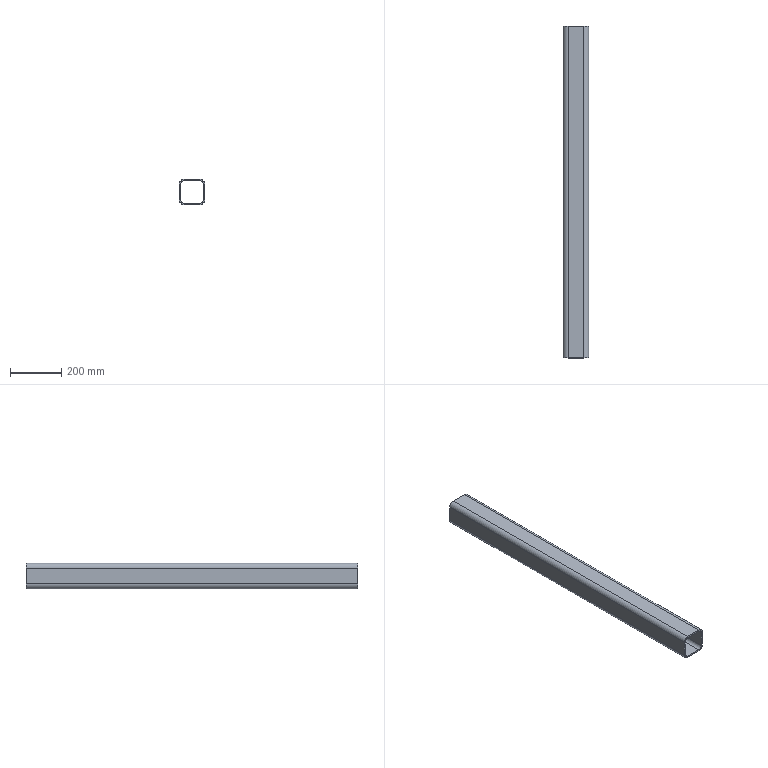Part | SolidWorks | features WeldMemberFeat 1, WeldmentFeature 1 | 1 solid | 18 faces | box 100 x 1293 x 100 mm | volume 2703104 mm3 | plane 10 | cylinder 8 | commonest cylinder face diameters 26.12 x4 38.12 x4
STEP:
#1=CARTESIAN_POINT('',(50.,1293.,30.94));
#2=VERTEX_POINT('',#1);
#3=CARTESIAN_POINT('',(30.94,1293.,50.));
#4=VERTEX_POINT('',#3);
#5=CARTESIAN_POINT('',(30.94,1293.,30.94));
#6=DIRECTION('',(0.,-1.,0.));
#7=DIRECTION('',(1.,0.,0.));
#8=AXIS2_PLACEMENT_3D('',#5,#6,#7);
#9=CIRCLE('',#8,19.06);
#10=EDGE_CURVE('',#2,#4,#9,.T.);
#11=ORIENTED_EDGE('',*,*,#10,.T.);
#12=CARTESIAN_POINT('',(30.94,0.,50.));
#13=VERTEX_POINT('',#12);
#14=CARTESIAN_POINT('',(30.94,0.,50.));
#15=DIRECTION('',(0.,1.,0.));
#16=VECTOR('',#15,1000.);
#17=LINE('',#14,#16);
#18=EDGE_CURVE('',#13,#4,#17,.T.);
#19=ORIENTED_EDGE('',*,*,#18,.F.);
#20=CARTESIAN_POINT('',(50.,0.,30.94));
#21=VERTEX_POINT('',#20);
#22=CARTESIAN_POINT('',(30.94,0.,30.94));
#23=DIRECTION('',(0.,-1.,0.));
#24=DIRECTION('',(1.,0.,0.));
#25=AXIS2_PLACEMENT_3D('',#22,#23,#24);
#26=CIRCLE('',#25,19.06);
#27=EDGE_CURVE('',#21,#13,#26,.T.);
#28=ORIENTED_EDGE('',*,*,#27,.F.);
#29=CARTESIAN_POINT('',(50.,0.,30.94));
#30=DIRECTION('',(0.,1.,0.));
#31=VECTOR('',#30,1000.);
#32=LINE('',#29,#31);
#33=EDGE_CURVE('',#21,#2,#32,.T.);
#34=ORIENTED_EDGE('',*,*,#33,.T.);
#35=EDGE_LOOP('',(#11,#19,#28,#34));
#36=FACE_OUTER_BOUND('',#35,.T.);
#37=CARTESIAN_POINT('',(30.94,0.,30.94));
#38=DIRECTION('',(0.,1.,0.));
#39=DIRECTION('',(-1.,0.,0.));
#40=AXIS2_PLACEMENT_3D('',#37,#38,#39);
#41=CYLINDRICAL_SURFACE('',#40,19.06);
#42=ADVANCED_FACE('',(#36),#41,.T.);
#43=CARTESIAN_POINT('',(-30.94,1293.,50.));
#44=VERTEX_POINT('',#43);
#45=CARTESIAN_POINT('',(30.94,1293.,50.));
#46=DIRECTION('',(-1.,0.,0.));
#47=VECTOR('',#46,1000.);
#48=LINE('',#45,#47);
#49=EDGE_CURVE('',#4,#44,#48,.T.);
#50=ORIENTED_EDGE('',*,*,#49,.T.);
#51=CARTESIAN_POINT('',(-30.94,0.,50.));
#52=VERTEX_POINT('',#51);
#53=CARTESIAN_POINT('',(-30.94,0.,50.));
#54=DIRECTION('',(0.,1.,0.));
#55=VECTOR('',#54,1000.);
#56=LINE('',#53,#55);
#57=EDGE_CURVE('',#52,#44,#56,.T.);
#58=ORIENTED_EDGE('',*,*,#57,.F.);
#59=CARTESIAN_POINT('',(30.94,0.,50.));
#60=DIRECTION('',(-1.,0.,0.));
#61=VECTOR('',#60,1000.);
#62=LINE('',#59,#61);
#63=EDGE_CURVE('',#13,#52,#62,.T.);
#64=ORIENTED_EDGE('',*,*,#63,.F.);
#65=ORIENTED_EDGE('',*,*,#18,.T.);
#66=EDGE_LOOP('',(#50,#58,#64,#65));
#67=FACE_OUTER_BOUND('',#66,.T.);
#68=CARTESIAN_POINT('',(30.94,0.,50.));
#69=DIRECTION('',(0.,0.,-1.));
#70=DIRECTION('',(-1.,0.,0.));
#71=AXIS2_PLACEMENT_3D('',#68,#69,#70);
#72=PLANE('',#71);
#73=ADVANCED_FACE('',(#67),#72,.F.);
#74=CARTESIAN_POINT('',(-50.,1293.,30.94));
#75=VERTEX_POINT('',#74);
#76=CARTESIAN_POINT('',(-30.94,1293.,30.94));
#77=DIRECTION('',(0.,-1.,0.));
#78=DIRECTION('',(1.,0.,0.));
#79=AXIS2_PLACEMENT_3D('',#76,#77,#78);
#80=CIRCLE('',#79,19.06);
#81=EDGE_CURVE('',#44,#75,#80,.T.);
#82=ORIENTED_EDGE('',*,*,#81,.T.);
#83=CARTESIAN_POINT('',(-50.,0.,30.94));
#84=VERTEX_POINT('',#83);
#85=CARTESIAN_POINT('',(-50.,0.,30.94));
#86=DIRECTION('',(0.,1.,0.));
#87=VECTOR('',#86,1000.);
#88=LINE('',#85,#87);
#89=EDGE_CURVE('',#84,#75,#88,.T.);
#90=ORIENTED_EDGE('',*,*,#89,.F.);
#91=CARTESIAN_POINT('',(-30.94,0.,30.94));
#92=DIRECTION('',(0.,-1.,0.));
#93=DIRECTION('',(1.,0.,0.));
#94=AXIS2_PLACEMENT_3D('',#91,#92,#93);
#95=CIRCLE('',#94,19.06);
#96=EDGE_CURVE('',#52,#84,#95,.T.);
#97=ORIENTED_EDGE('',*,*,#96,.F.);
#98=ORIENTED_EDGE('',*,*,#57,.T.);
#99=EDGE_LOOP('',(#82,#90,#97,#98));
#100=FACE_OUTER_BOUND('',#99,.T.);
#101=CARTESIAN_POINT('',(-30.94,0.,30.94));
#102=DIRECTION('',(0.,1.,0.));
#103=DIRECTION('',(-1.,0.,0.));
#104=AXIS2_PLACEMENT_3D('',#101,#102,#103);
#105=CYLINDRICAL_SURFACE('',#104,19.06);
#106=ADVANCED_FACE('',(#100),#105,.T.);
#107=CARTESIAN_POINT('',(-50.,1293.,-30.94));
#108=VERTEX_POINT('',#107);
#109=CARTESIAN_POINT('',(-50.,1293.,-30.94));
#110=DIRECTION('',(0.,0.,-1.));
#111=VECTOR('',#110,1000.);
#112=LINE('',#109,#111);
#113=EDGE_CURVE('',#75,#108,#112,.T.);
#114=ORIENTED_EDGE('',*,*,#113,.T.);
#115=CARTESIAN_POINT('',(-50.,0.,-30.94));
#116=VERTEX_POINT('',#115);
#117=CARTESIAN_POINT('',(-50.,0.,-30.94));
#118=DIRECTION('',(0.,1.,0.));
#119=VECTOR('',#118,1000.);
#120=LINE('',#117,#119);
#121=EDGE_CURVE('',#116,#108,#120,.T.);
#122=ORIENTED_EDGE('',*,*,#121,.F.);
#123=CARTESIAN_POINT('',(-50.,0.,-30.94));
#124=DIRECTION('',(0.,0.,-1.));
#125=VECTOR('',#124,1000.);
#126=LINE('',#123,#125);
#127=EDGE_CURVE('',#84,#116,#126,.T.);
#128=ORIENTED_EDGE('',*,*,#127,.F.);
#129=ORIENTED_EDGE('',*,*,#89,.T.);
#130=EDGE_LOOP('',(#114,#122,#128,#129));
#131=FACE_OUTER_BOUND('',#130,.T.);
#132=CARTESIAN_POINT('',(-50.,0.,-30.94));
#133=DIRECTION('',(1.,0.,0.));
#134=DIRECTION('',(0.,0.,-1.));
#135=AXIS2_PLACEMENT_3D('',#132,#133,#134);
#136=PLANE('',#135);
#137=ADVANCED_FACE('',(#131),#136,.F.);
#138=CARTESIAN_POINT('',(-30.94,1293.,-50.));
#139=VERTEX_POINT('',#138);
#140=CARTESIAN_POINT('',(-30.94,1293.,-30.94));
#141=DIRECTION('',(0.,-1.,0.));
#142=DIRECTION('',(1.,0.,0.));
#143=AXIS2_PLACEMENT_3D('',#140,#141,#142);
#144=CIRCLE('',#143,19.06);
#145=EDGE_CURVE('',#108,#139,#144,.T.);
#146=ORIENTED_EDGE('',*,*,#145,.T.);
#147=CARTESIAN_POINT('',(-30.94,0.,-50.));
#148=VERTEX_POINT('',#147);
#149=CARTESIAN_POINT('',(-30.94,0.,-50.));
#150=DIRECTION('',(0.,1.,0.));
#151=VECTOR('',#150,1000.);
#152=LINE('',#149,#151);
#153=EDGE_CURVE('',#148,#139,#152,.T.);
#154=ORIENTED_EDGE('',*,*,#153,.F.);
#155=CARTESIAN_POINT('',(-30.94,0.,-30.94));
#156=DIRECTION('',(0.,-1.,0.));
#157=DIRECTION('',(1.,0.,0.));
#158=AXIS2_PLACEMENT_3D('',#155,#156,#157);
#159=CIRCLE('',#158,19.06);
#160=EDGE_CURVE('',#116,#148,#159,.T.);
#161=ORIENTED_EDGE('',*,*,#160,.F.);
#162=ORIENTED_EDGE('',*,*,#121,.T.);
#163=EDGE_LOOP('',(#146,#154,#161,#162));
#164=FACE_OUTER_BOUND('',#163,.T.);
#165=CARTESIAN_POINT('',(-30.94,0.,-30.94));
#166=DIRECTION('',(0.,1.,0.));
#167=DIRECTION('',(-1.,0.,0.));
#168=AXIS2_PLACEMENT_3D('',#165,#166,#167);
#169=CYLINDRICAL_SURFACE('',#168,19.06);
#170=ADVANCED_FACE('',(#164),#169,.T.);
#171=CARTESIAN_POINT('',(30.94,1293.,-50.));
#172=VERTEX_POINT('',#171);
#173=CARTESIAN_POINT('',(-30.94,1293.,-50.));
#174=DIRECTION('',(1.,0.,0.));
#175=VECTOR('',#174,1000.);
#176=LINE('',#173,#175);
#177=EDGE_CURVE('',#139,#172,#176,.T.);
#178=ORIENTED_EDGE('',*,*,#177,.T.);
#179=CARTESIAN_POINT('',(30.94,0.,-50.));
#180=VERTEX_POINT('',#179);
#181=CARTESIAN_POINT('',(30.94,0.,-50.));
#182=DIRECTION('',(0.,1.,0.));
#183=VECTOR('',#182,1000.);
#184=LINE('',#181,#183);
#185=EDGE_CURVE('',#180,#172,#184,.T.);
#186=ORIENTED_EDGE('',*,*,#185,.F.);
#187=CARTESIAN_POINT('',(-30.94,0.,-50.));
#188=DIRECTION('',(1.,0.,0.));
#189=VECTOR('',#188,1000.);
#190=LINE('',#187,#189);
#191=EDGE_CURVE('',#148,#180,#190,.T.);
#192=ORIENTED_EDGE('',*,*,#191,.F.);
#193=ORIENTED_EDGE('',*,*,#153,.T.);
#194=EDGE_LOOP('',(#178,#186,#192,#193));
#195=FACE_OUTER_BOUND('',#194,.T.);
#196=CARTESIAN_POINT('',(-30.94,0.,-50.));
#197=DIRECTION('',(0.,0.,1.));
#198=DIRECTION('',(1.,0.,0.));
#199=AXIS2_PLACEMENT_3D('',#196,#197,#198);
#200=PLANE('',#199);
#201=ADVANCED_FACE('',(#195),#200,.F.);
#202=CARTESIAN_POINT('',(50.,1293.,-30.94));
#203=VERTEX_POINT('',#202);
#204=CARTESIAN_POINT('',(30.94,1293.,-30.94));
#205=DIRECTION('',(0.,-1.,0.));
#206=DIRECTION('',(1.,0.,0.));
#207=AXIS2_PLACEMENT_3D('',#204,#205,#206);
#208=CIRCLE('',#207,19.06);
#209=EDGE_CURVE('',#172,#203,#208,.T.);
#210=ORIENTED_EDGE('',*,*,#209,.T.);
#211=CARTESIAN_POINT('',(50.,0.,-30.94));
#212=VERTEX_POINT('',#211);
#213=CARTESIAN_POINT('',(50.,0.,-30.94));
#214=DIRECTION('',(0.,1.,0.));
#215=VECTOR('',#214,1000.);
#216=LINE('',#213,#215);
#217=EDGE_CURVE('',#212,#203,#216,.T.);
#218=ORIENTED_EDGE('',*,*,#217,.F.);
#219=CARTESIAN_POINT('',(30.94,0.,-30.94));
#220=DIRECTION('',(0.,-1.,0.));
#221=DIRECTION('',(1.,0.,0.));
#222=AXIS2_PLACEMENT_3D('',#219,#220,#221);
#223=CIRCLE('',#222,19.06);
#224=EDGE_CURVE('',#180,#212,#223,.T.);
#225=ORIENTED_EDGE('',*,*,#224,.F.);
#226=ORIENTED_EDGE('',*,*,#185,.T.);
#227=EDGE_LOOP('',(#210,#218,#225,#226));
#228=FACE_OUTER_BOUND('',#227,.T.);
#229=CARTESIAN_POINT('',(30.94,0.,-30.94));
#230=DIRECTION('',(0.,1.,0.));
#231=DIRECTION('',(-1.,0.,0.));
#232=AXIS2_PLACEMENT_3D('',#229,#230,#231);
#233=CYLINDRICAL_SURFACE('',#232,19.06);
#234=ADVANCED_FACE('',(#228),#233,.T.);
#235=CARTESIAN_POINT('',(-30.94,1293.,44.));
#236=VERTEX_POINT('',#235);
#237=CARTESIAN_POINT('',(-44.,1293.,30.94));
#238=VERTEX_POINT('',#237);
#239=CARTESIAN_POINT('',(-30.94,1293.,30.94));
#240=DIRECTION('',(0.,-1.,0.));
#241=DIRECTION('',(1.,0.,0.));
#242=AXIS2_PLACEMENT_3D('',#239,#240,#241);
#243=CIRCLE('',#242,13.06);
#244=EDGE_CURVE('',#236,#238,#243,.T.);
#245=ORIENTED_EDGE('',*,*,#244,.F.);
#246=CARTESIAN_POINT('',(-30.94,0.,44.));
#247=VERTEX_POINT('',#246);
#248=CARTESIAN_POINT('',(-30.94,0.,44.));
#249=DIRECTION('',(0.,1.,0.));
#250=VECTOR('',#249,1000.);
#251=LINE('',#248,#250);
#252=EDGE_CURVE('',#247,#236,#251,.T.);
#253=ORIENTED_EDGE('',*,*,#252,.F.);
#254=CARTESIAN_POINT('',(-44.,0.,30.94));
#255=VERTEX_POINT('',#254);
#256=CARTESIAN_POINT('',(-30.94,0.,30.94));
#257=DIRECTION('',(0.,-1.,0.));
#258=DIRECTION('',(1.,0.,0.));
#259=AXIS2_PLACEMENT_3D('',#256,#257,#258);
#260=CIRCLE('',#259,13.06);
#261=EDGE_CURVE('',#247,#255,#260,.T.);
#262=ORIENTED_EDGE('',*,*,#261,.T.);
#263=CARTESIAN_POINT('',(-44.,0.,30.94));
#264=DIRECTION('',(0.,1.,0.));
#265=VECTOR('',#264,1000.);
#266=LINE('',#263,#265);
#267=EDGE_CURVE('',#255,#238,#266,.T.);
#268=ORIENTED_EDGE('',*,*,#267,.T.);
#269=EDGE_LOOP('',(#245,#253,#262,#268));
#270=FACE_OUTER_BOUND('',#269,.T.);
#271=CARTESIAN_POINT('',(-30.94,0.,30.94));
#272=DIRECTION('',(0.,1.,0.));
#273=DIRECTION('',(-1.,0.,0.));
#274=AXIS2_PLACEMENT_3D('',#271,#272,#273);
#275=CYLINDRICAL_SURFACE('',#274,13.06);
#276=ADVANCED_FACE('',(#270),#275,.F.);
#277=CARTESIAN_POINT('',(30.94,1293.,44.));
#278=VERTEX_POINT('',#277);
#279=CARTESIAN_POINT('',(30.94,1293.,44.));
#280=DIRECTION('',(-1.,0.,0.));
#281=VECTOR('',#280,1000.);
#282=LINE('',#279,#281);
#283=EDGE_CURVE('',#278,#236,#282,.T.);
#284=ORIENTED_EDGE('',*,*,#283,.F.);
#285=CARTESIAN_POINT('',(30.94,0.,44.));
#286=VERTEX_POINT('',#285);
#287=CARTESIAN_POINT('',(30.94,0.,44.));
#288=DIRECTION('',(0.,1.,0.));
#289=VECTOR('',#288,1000.);
#290=LINE('',#287,#289);
#291=EDGE_CURVE('',#286,#278,#290,.T.);
#292=ORIENTED_EDGE('',*,*,#291,.F.);
#293=CARTESIAN_POINT('',(30.94,0.,44.));
#294=DIRECTION('',(-1.,0.,0.));
#295=VECTOR('',#294,1000.);
#296=LINE('',#293,#295);
#297=EDGE_CURVE('',#286,#247,#296,.T.);
#298=ORIENTED_EDGE('',*,*,#297,.T.);
#299=ORIENTED_EDGE('',*,*,#252,.T.);
#300=EDGE_LOOP('',(#284,#292,#298,#299));
#301=FACE_OUTER_BOUND('',#300,.T.);
#302=CARTESIAN_POINT('',(30.94,0.,44.));
#303=DIRECTION('',(0.,0.,-1.));
#304=DIRECTION('',(-1.,0.,0.));
#305=AXIS2_PLACEMENT_3D('',#302,#303,#304);
#306=PLANE('',#305);
#307=ADVANCED_FACE('',(#301),#306,.T.);
#308=CARTESIAN_POINT('',(44.,1293.,30.94));
#309=VERTEX_POINT('',#308);
#310=CARTESIAN_POINT('',(30.94,1293.,30.94));
#311=DIRECTION('',(0.,-1.,0.));
#312=DIRECTION('',(1.,0.,0.));
#313=AXIS2_PLACEMENT_3D('',#310,#311,#312);
#314=CIRCLE('',#313,13.06);
#315=EDGE_CURVE('',#309,#278,#314,.T.);
#316=ORIENTED_EDGE('',*,*,#315,.F.);
#317=CARTESIAN_POINT('',(44.,0.,30.94));
#318=VERTEX_POINT('',#317);
#319=CARTESIAN_POINT('',(44.,0.,30.94));
#320=DIRECTION('',(0.,1.,0.));
#321=VECTOR('',#320,1000.);
#322=LINE('',#319,#321);
#323=EDGE_CURVE('',#318,#309,#322,.T.);
#324=ORIENTED_EDGE('',*,*,#323,.F.);
#325=CARTESIAN_POINT('',(30.94,0.,30.94));
#326=DIRECTION('',(0.,-1.,0.));
#327=DIRECTION('',(1.,0.,0.));
#328=AXIS2_PLACEMENT_3D('',#325,#326,#327);
#329=CIRCLE('',#328,13.06);
#330=EDGE_CURVE('',#318,#286,#329,.T.);
#331=ORIENTED_EDGE('',*,*,#330,.T.);
#332=ORIENTED_EDGE('',*,*,#291,.T.);
#333=EDGE_LOOP('',(#316,#324,#331,#332));
#334=FACE_OUTER_BOUND('',#333,.T.);
#335=CARTESIAN_POINT('',(30.94,0.,30.94));
#336=DIRECTION('',(0.,1.,0.));
#337=DIRECTION('',(-1.,0.,0.));
#338=AXIS2_PLACEMENT_3D('',#335,#336,#337);
#339=CYLINDRICAL_SURFACE('',#338,13.06);
#340=ADVANCED_FACE('',(#334),#339,.F.);
#341=CARTESIAN_POINT('',(44.,1293.,-30.94));
#342=VERTEX_POINT('',#341);
#343=CARTESIAN_POINT('',(44.,1293.,30.94));
#344=DIRECTION('',(0.,0.,1.));
#345=VECTOR('',#344,1000.);
#346=LINE('',#343,#345);
#347=EDGE_CURVE('',#342,#309,#346,.T.);
#348=ORIENTED_EDGE('',*,*,#347,.F.);
#349=CARTESIAN_POINT('',(44.,0.,-30.94));
#350=VERTEX_POINT('',#349);
#351=CARTESIAN_POINT('',(44.,0.,-30.94));
#352=DIRECTION('',(0.,1.,0.));
#353=VECTOR('',#352,1000.);
#354=LINE('',#351,#353);
#355=EDGE_CURVE('',#350,#342,#354,.T.);
#356=ORIENTED_EDGE('',*,*,#355,.F.);
#357=CARTESIAN_POINT('',(44.,0.,30.94));
#358=DIRECTION('',(0.,0.,1.));
#359=VECTOR('',#358,1000.);
#360=LINE('',#357,#359);
#361=EDGE_CURVE('',#350,#318,#360,.T.);
#362=ORIENTED_EDGE('',*,*,#361,.T.);
#363=ORIENTED_EDGE('',*,*,#323,.T.);
#364=EDGE_LOOP('',(#348,#356,#362,#363));
#365=FACE_OUTER_BOUND('',#364,.T.);
#366=CARTESIAN_POINT('',(44.,0.,30.94));
#367=DIRECTION('',(-1.,0.,0.));
#368=DIRECTION('',(0.,-1.,0.));
#369=AXIS2_PLACEMENT_3D('',#366,#367,#368);
#370=PLANE('',#369);
#371=ADVANCED_FACE('',(#365),#370,.T.);
#372=CARTESIAN_POINT('',(30.94,1293.,-44.));
#373=VERTEX_POINT('',#372);
#374=CARTESIAN_POINT('',(30.94,1293.,-30.94));
#375=DIRECTION('',(0.,-1.,0.));
#376=DIRECTION('',(1.,0.,0.));
#377=AXIS2_PLACEMENT_3D('',#374,#375,#376);
#378=CIRCLE('',#377,13.06);
#379=EDGE_CURVE('',#373,#342,#378,.T.);
#380=ORIENTED_EDGE('',*,*,#379,.F.);
#381=CARTESIAN_POINT('',(30.94,0.,-44.));
#382=VERTEX_POINT('',#381);
#383=CARTESIAN_POINT('',(30.94,0.,-44.));
#384=DIRECTION('',(0.,1.,0.));
#385=VECTOR('',#384,1000.);
#386=LINE('',#383,#385);
#387=EDGE_CURVE('',#382,#373,#386,.T.);
#388=ORIENTED_EDGE('',*,*,#387,.F.);
#389=CARTESIAN_POINT('',(30.94,0.,-30.94));
#390=DIRECTION('',(0.,-1.,0.));
#391=DIRECTION('',(1.,0.,0.));
#392=AXIS2_PLACEMENT_3D('',#389,#390,#391);
#393=CIRCLE('',#392,13.06);
#394=EDGE_CURVE('',#382,#350,#393,.T.);
#395=ORIENTED_EDGE('',*,*,#394,.T.);
#396=ORIENTED_EDGE('',*,*,#355,.T.);
#397=EDGE_LOOP('',(#380,#388,#395,#396));
#398=FACE_OUTER_BOUND('',#397,.T.);
#399=CARTESIAN_POINT('',(30.94,0.,-30.94));
#400=DIRECTION('',(0.,1.,0.));
#401=DIRECTION('',(-1.,0.,0.));
#402=AXIS2_PLACEMENT_3D('',#399,#400,#401);
#403=CYLINDRICAL_SURFACE('',#402,13.06);
#404=ADVANCED_FACE('',(#398),#403,.F.);
#405=CARTESIAN_POINT('',(-30.94,1293.,-44.));
#406=VERTEX_POINT('',#405);
#407=CARTESIAN_POINT('',(-30.94,1293.,-44.));
#408=DIRECTION('',(1.,0.,0.));
#409=VECTOR('',#408,1000.);
#410=LINE('',#407,#409);
#411=EDGE_CURVE('',#406,#373,#410,.T.);
#412=ORIENTED_EDGE('',*,*,#411,.F.);
#413=CARTESIAN_POINT('',(-30.94,0.,-44.));
#414=VERTEX_POINT('',#413);
#415=CARTESIAN_POINT('',(-30.94,0.,-44.));
#416=DIRECTION('',(0.,1.,0.));
#417=VECTOR('',#416,1000.);
#418=LINE('',#415,#417);
#419=EDGE_CURVE('',#414,#406,#418,.T.);
#420=ORIENTED_EDGE('',*,*,#419,.F.);
#421=CARTESIAN_POINT('',(-30.94,0.,-44.));
#422=DIRECTION('',(1.,0.,0.));
#423=VECTOR('',#422,1000.);
#424=LINE('',#421,#423);
#425=EDGE_CURVE('',#414,#382,#424,.T.);
#426=ORIENTED_EDGE('',*,*,#425,.T.);
#427=ORIENTED_EDGE('',*,*,#387,.T.);
#428=EDGE_LOOP('',(#412,#420,#426,#427));
#429=FACE_OUTER_BOUND('',#428,.T.);
#430=CARTESIAN_POINT('',(-30.94,0.,-44.));
#431=DIRECTION('',(0.,0.,1.));
#432=DIRECTION('',(1.,0.,0.));
#433=AXIS2_PLACEMENT_3D('',#430,#431,#432);
#434=PLANE('',#433);
#435=ADVANCED_FACE('',(#429),#434,.T.);
#436=CARTESIAN_POINT('',(-44.,1293.,-30.94));
#437=VERTEX_POINT('',#436);
#438=CARTESIAN_POINT('',(-30.94,1293.,-30.94));
#439=DIRECTION('',(0.,-1.,0.));
#440=DIRECTION('',(1.,0.,0.));
#441=AXIS2_PLACEMENT_3D('',#438,#439,#440);
#442=CIRCLE('',#441,13.06);
#443=EDGE_CURVE('',#437,#406,#442,.T.);
#444=ORIENTED_EDGE('',*,*,#443,.F.);
#445=CARTESIAN_POINT('',(-44.,0.,-30.94));
#446=VERTEX_POINT('',#445);
#447=CARTESIAN_POINT('',(-44.,0.,-30.94));
#448=DIRECTION('',(0.,1.,0.));
#449=VECTOR('',#448,1000.);
#450=LINE('',#447,#449);
#451=EDGE_CURVE('',#446,#437,#450,.T.);
#452=ORIENTED_EDGE('',*,*,#451,.F.);
#453=CARTESIAN_POINT('',(-30.94,0.,-30.94));
#454=DIRECTION('',(0.,-1.,0.));
#455=DIRECTION('',(1.,0.,0.));
#456=AXIS2_PLACEMENT_3D('',#453,#454,#455);
#457=CIRCLE('',#456,13.06);
#458=EDGE_CURVE('',#446,#414,#457,.T.);
#459=ORIENTED_EDGE('',*,*,#458,.T.);
#460=ORIENTED_EDGE('',*,*,#419,.T.);
#461=EDGE_LOOP('',(#444,#452,#459,#460));
#462=FACE_OUTER_BOUND('',#461,.T.);
#463=CARTESIAN_POINT('',(-30.94,0.,-30.94));
#464=DIRECTION('',(0.,1.,0.));
#465=DIRECTION('',(-1.,0.,0.));
#466=AXIS2_PLACEMENT_3D('',#463,#464,#465);
#467=CYLINDRICAL_SURFACE('',#466,13.06);
#468=ADVANCED_FACE('',(#462),#467,.F.);
#469=CARTESIAN_POINT('',(-44.,1293.,-30.94));
#470=DIRECTION('',(0.,0.,-1.));
#471=VECTOR('',#470,1000.);
#472=LINE('',#469,#471);
#473=EDGE_CURVE('',#238,#437,#472,.T.);
#474=ORIENTED_EDGE('',*,*,#473,.F.);
#475=ORIENTED_EDGE('',*,*,#267,.F.);
#476=CARTESIAN_POINT('',(-44.,0.,-30.94));
#477=DIRECTION('',(0.,0.,-1.));
#478=VECTOR('',#477,1000.);
#479=LINE('',#476,#478);
#480=EDGE_CURVE('',#255,#446,#479,.T.);
#481=ORIENTED_EDGE('',*,*,#480,.T.);
#482=ORIENTED_EDGE('',*,*,#451,.T.);
#483=EDGE_LOOP('',(#474,#475,#481,#482));
#484=FACE_OUTER_BOUND('',#483,.T.);
#485=CARTESIAN_POINT('',(-44.,0.,-30.94));
#486=DIRECTION('',(1.,0.,0.));
#487=DIRECTION('',(0.,0.,-1.));
#488=AXIS2_PLACEMENT_3D('',#485,#486,#487);
#489=PLANE('',#488);
#490=ADVANCED_FACE('',(#484),#489,.T.);
#491=CARTESIAN_POINT('',(50.,1293.,30.94));
#492=DIRECTION('',(0.,0.,1.));
#493=VECTOR('',#492,1000.);
#494=LINE('',#491,#493);
#495=EDGE_CURVE('',#203,#2,#494,.T.);
#496=ORIENTED_EDGE('',*,*,#495,.T.);
#497=ORIENTED_EDGE('',*,*,#33,.F.);
#498=CARTESIAN_POINT('',(50.,0.,30.94));
#499=DIRECTION('',(0.,0.,1.));
#500=VECTOR('',#499,1000.);
#501=LINE('',#498,#500);
#502=EDGE_CURVE('',#212,#21,#501,.T.);
#503=ORIENTED_EDGE('',*,*,#502,.F.);
#504=ORIENTED_EDGE('',*,*,#217,.T.);
#505=EDGE_LOOP('',(#496,#497,#503,#504));
#506=FACE_OUTER_BOUND('',#505,.T.);
#507=CARTESIAN_POINT('',(50.,0.,30.94));
#508=DIRECTION('',(-1.,0.,0.));
#509=DIRECTION('',(0.,-1.,0.));
#510=AXIS2_PLACEMENT_3D('',#507,#508,#509);
#511=PLANE('',#510);
#512=ADVANCED_FACE('',(#506),#511,.F.);
#513=ORIENTED_EDGE('',*,*,#261,.F.);
#514=ORIENTED_EDGE('',*,*,#297,.F.);
#515=ORIENTED_EDGE('',*,*,#330,.F.);
#516=ORIENTED_EDGE('',*,*,#361,.F.);
#517=ORIENTED_EDGE('',*,*,#394,.F.);
#518=ORIENTED_EDGE('',*,*,#425,.F.);
#519=ORIENTED_EDGE('',*,*,#458,.F.);
#520=ORIENTED_EDGE('',*,*,#480,.F.);
#521=EDGE_LOOP('',(#513,#514,#515,#516,#517,#518,#519,#520));
#522=FACE_BOUND('',#521,.T.);
#523=ORIENTED_EDGE('',*,*,#27,.T.);
#524=ORIENTED_EDGE('',*,*,#63,.T.);
#525=ORIENTED_EDGE('',*,*,#96,.T.);
#526=ORIENTED_EDGE('',*,*,#127,.T.);
#527=ORIENTED_EDGE('',*,*,#160,.T.);
#528=ORIENTED_EDGE('',*,*,#191,.T.);
#529=ORIENTED_EDGE('',*,*,#224,.T.);
#530=ORIENTED_EDGE('',*,*,#502,.T.);
#531=EDGE_LOOP('',(#523,#524,#525,#526,#527,#528,#529,#530));
#532=FACE_OUTER_BOUND('',#531,.T.);
#533=CARTESIAN_POINT('',(30.94,0.,30.94));
#534=DIRECTION('',(0.,-1.,0.));
#535=DIRECTION('',(1.,0.,0.));
#536=AXIS2_PLACEMENT_3D('',#533,#534,#535);
#537=PLANE('',#536);
#538=ADVANCED_FACE('',(#522,#532),#537,.T.);
#539=ORIENTED_EDGE('',*,*,#244,.T.);
#540=ORIENTED_EDGE('',*,*,#473,.T.);
#541=ORIENTED_EDGE('',*,*,#443,.T.);
#542=ORIENTED_EDGE('',*,*,#411,.T.);
#543=ORIENTED_EDGE('',*,*,#379,.T.);
#544=ORIENTED_EDGE('',*,*,#347,.T.);
#545=ORIENTED_EDGE('',*,*,#315,.T.);
#546=ORIENTED_EDGE('',*,*,#283,.T.);
#547=EDGE_LOOP('',(#539,#540,#541,#542,#543,#544,#545,#546));
#548=FACE_BOUND('',#547,.T.);
#549=ORIENTED_EDGE('',*,*,#10,.F.);
#550=ORIENTED_EDGE('',*,*,#495,.F.);
#551=ORIENTED_EDGE('',*,*,#209,.F.);
#552=ORIENTED_EDGE('',*,*,#177,.F.);
#553=ORIENTED_EDGE('',*,*,#145,.F.);
#554=ORIENTED_EDGE('',*,*,#113,.F.);
#555=ORIENTED_EDGE('',*,*,#81,.F.);
#556=ORIENTED_EDGE('',*,*,#49,.F.);
#557=EDGE_LOOP('',(#549,#550,#551,#552,#553,#554,#555,#556));
#558=FACE_OUTER_BOUND('',#557,.T.);
#559=CARTESIAN_POINT('',(30.94,1293.,30.94));
#560=DIRECTION('',(0.,-1.,0.));
#561=DIRECTION('',(1.,0.,0.));
#562=AXIS2_PLACEMENT_3D('',#559,#560,#561);
#563=PLANE('',#562);
#564=ADVANCED_FACE('',(#548,#558),#563,.F.);
#565=CLOSED_SHELL('',(#42,#73,#106,#137,#170,#201,#234,#276,#307,#340,#371,#404,#435,#468,#490,#512,#538,#564));
#566=MANIFOLD_SOLID_BREP('',#565);
#567=CARTESIAN_POINT('',(0.,0.,0.));
#568=DIRECTION('',(0.,0.,1.));
#569=DIRECTION('',(1.,0.,0.));
#570=AXIS2_PLACEMENT_3D('',#567,#568,#569);
#571=(LENGTH_UNIT()NAMED_UNIT(*)SI_UNIT(.MILLI.,.METRE.));
#572=UNCERTAINTY_MEASURE_WITH_UNIT(LENGTH_MEASURE(0.00001),#571,'','');
#573=(NAMED_UNIT(*)PLANE_ANGLE_UNIT()SI_UNIT($,.RADIAN.));
#574=(NAMED_UNIT(*)SI_UNIT($,.STERADIAN.)SOLID_ANGLE_UNIT());
#575=(GEOMETRIC_REPRESENTATION_CONTEXT(3)GLOBAL_UNCERTAINTY_ASSIGNED_CONTEXT((#572))GLOBAL_UNIT_ASSIGNED_CONTEXT((#571,#573,#574))REPRESENTATION_CONTEXT('',''));
#576=ADVANCED_BREP_SHAPE_REPRESENTATION('',(#566,#570),#575);